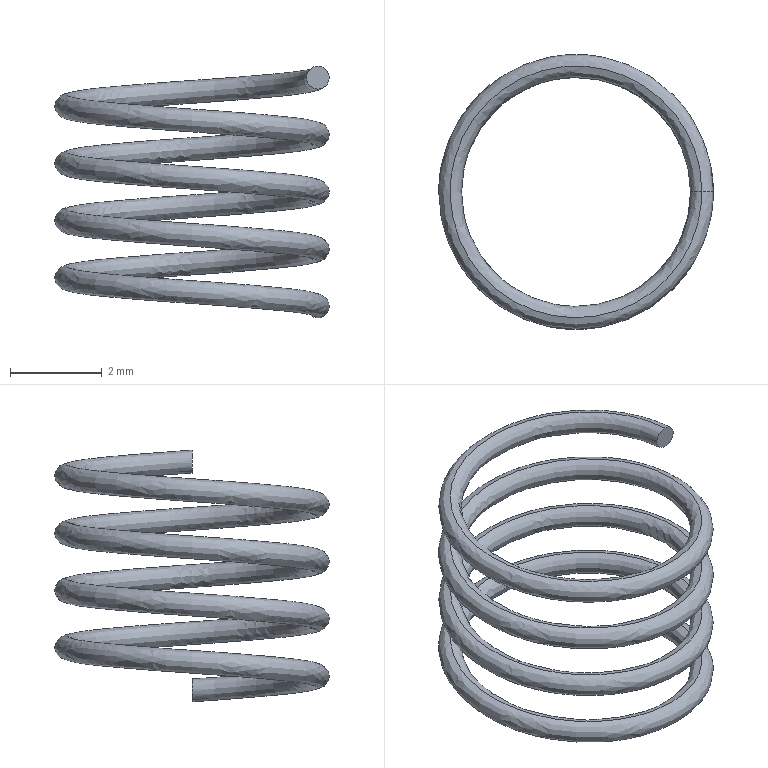Part | SolidWorks | features Helix 1, Sweep 1 | 1 solid | 4 faces | box 6 x 6 x 5.5 mm | volume 13.577 mm3 | spline 2 | plane 2